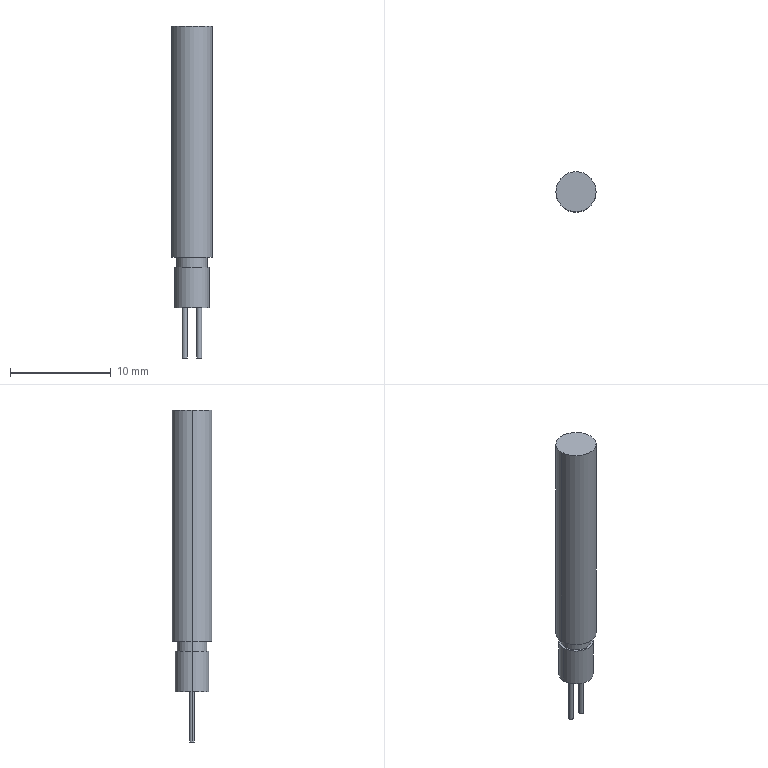Part | NX | 1 solid | 16 faces | box 4 x 4 x 33 mm | volume 334.375 mm3 | cylinder 10 | plane 6 | commonest cylinder face diameters 0.5 x4 3 x2 3.4 x2 4 x2
STEP:
#1=CARTESIAN_POINT('',(0.46,0.,-10.));
#2=VERTEX_POINT('',#1);
#3=CARTESIAN_POINT('',(0.96,0.,-10.));
#4=VERTEX_POINT('',#3);
#5=CARTESIAN_POINT('',(0.71,0.,-10.));
#6=DIRECTION('',(0.,0.,-1.));
#7=DIRECTION('',(-1.,0.,0.));
#8=AXIS2_PLACEMENT_3D('',#5,#6,#7);
#9=CIRCLE('',#8,0.25);
#10=EDGE_CURVE('',#2,#4,#9,.T.);
#11=ORIENTED_EDGE('',*,*,#10,.F.);
#12=CARTESIAN_POINT('',(0.46,0.,-5.));
#13=VERTEX_POINT('',#12);
#14=CARTESIAN_POINT('',(0.46,0.,-10.));
#15=DIRECTION('',(0.,0.,1.));
#16=VECTOR('',#15,1000.);
#17=LINE('',#14,#16);
#18=EDGE_CURVE('',#2,#13,#17,.T.);
#19=ORIENTED_EDGE('',*,*,#18,.T.);
#20=CARTESIAN_POINT('',(0.96,0.,-5.));
#21=VERTEX_POINT('',#20);
#22=CARTESIAN_POINT('',(0.71,0.,-5.));
#23=DIRECTION('',(0.,0.,-1.));
#24=DIRECTION('',(1.,0.,0.));
#25=AXIS2_PLACEMENT_3D('',#22,#23,#24);
#26=CIRCLE('',#25,0.25);
#27=EDGE_CURVE('',#13,#21,#26,.T.);
#28=ORIENTED_EDGE('',*,*,#27,.T.);
#29=CARTESIAN_POINT('',(0.96,0.,-10.));
#30=DIRECTION('',(0.,0.,1.));
#31=VECTOR('',#30,1000.);
#32=LINE('',#29,#31);
#33=EDGE_CURVE('',#4,#21,#32,.T.);
#34=ORIENTED_EDGE('',*,*,#33,.F.);
#35=EDGE_LOOP('',(#11,#19,#28,#34));
#36=FACE_BOUND('',#35,.T.);
#37=CARTESIAN_POINT('',(0.71,0.,-10.));
#38=DIRECTION('',(0.,0.,1.));
#39=DIRECTION('',(1.,0.,0.));
#40=AXIS2_PLACEMENT_3D('',#37,#38,#39);
#41=CYLINDRICAL_SURFACE('',#40,0.25);
#42=ADVANCED_FACE('',(#36),#41,.T.);
#43=CARTESIAN_POINT('',(-0.46,0.,-10.));
#44=VERTEX_POINT('',#43);
#45=CARTESIAN_POINT('',(-0.96,0.,-10.));
#46=VERTEX_POINT('',#45);
#47=CARTESIAN_POINT('',(-0.71,0.,-10.));
#48=DIRECTION('',(0.,0.,-1.));
#49=DIRECTION('',(1.,0.,0.));
#50=AXIS2_PLACEMENT_3D('',#47,#48,#49);
#51=CIRCLE('',#50,0.25);
#52=EDGE_CURVE('',#44,#46,#51,.T.);
#53=ORIENTED_EDGE('',*,*,#52,.F.);
#54=CARTESIAN_POINT('',(-0.46,0.,-5.));
#55=VERTEX_POINT('',#54);
#56=CARTESIAN_POINT('',(-0.46,0.,-10.));
#57=DIRECTION('',(0.,0.,1.));
#58=VECTOR('',#57,1000.);
#59=LINE('',#56,#58);
#60=EDGE_CURVE('',#44,#55,#59,.T.);
#61=ORIENTED_EDGE('',*,*,#60,.T.);
#62=CARTESIAN_POINT('',(-0.96,0.,-5.));
#63=VERTEX_POINT('',#62);
#64=CARTESIAN_POINT('',(-0.71,0.,-5.));
#65=DIRECTION('',(0.,0.,-1.));
#66=DIRECTION('',(1.,0.,0.));
#67=AXIS2_PLACEMENT_3D('',#64,#65,#66);
#68=CIRCLE('',#67,0.25);
#69=EDGE_CURVE('',#55,#63,#68,.T.);
#70=ORIENTED_EDGE('',*,*,#69,.T.);
#71=CARTESIAN_POINT('',(-0.96,0.,-10.));
#72=DIRECTION('',(0.,0.,1.));
#73=VECTOR('',#72,1000.);
#74=LINE('',#71,#73);
#75=EDGE_CURVE('',#46,#63,#74,.T.);
#76=ORIENTED_EDGE('',*,*,#75,.F.);
#77=EDGE_LOOP('',(#53,#61,#70,#76));
#78=FACE_BOUND('',#77,.T.);
#79=CARTESIAN_POINT('',(-0.71,0.,-10.));
#80=DIRECTION('',(0.,0.,1.));
#81=DIRECTION('',(1.,0.,0.));
#82=AXIS2_PLACEMENT_3D('',#79,#80,#81);
#83=CYLINDRICAL_SURFACE('',#82,0.25);
#84=ADVANCED_FACE('',(#78),#83,.T.);
#85=CARTESIAN_POINT('',(1.7,0.,-1.));
#86=VERTEX_POINT('',#85);
#87=CARTESIAN_POINT('',(-1.7,0.,-1.));
#88=VERTEX_POINT('',#87);
#89=CARTESIAN_POINT('',(0.,0.,-1.));
#90=DIRECTION('',(0.,0.,-1.));
#91=DIRECTION('',(-1.,0.,0.));
#92=AXIS2_PLACEMENT_3D('',#89,#90,#91);
#93=CIRCLE('',#92,1.7);
#94=EDGE_CURVE('',#86,#88,#93,.T.);
#95=ORIENTED_EDGE('',*,*,#94,.T.);
#96=CARTESIAN_POINT('',(-1.7,0.,-5.));
#97=VERTEX_POINT('',#96);
#98=CARTESIAN_POINT('',(-1.7,0.,-5.));
#99=DIRECTION('',(0.,0.,1.));
#100=VECTOR('',#99,1000.);
#101=LINE('',#98,#100);
#102=EDGE_CURVE('',#97,#88,#101,.T.);
#103=ORIENTED_EDGE('',*,*,#102,.F.);
#104=CARTESIAN_POINT('',(1.7,0.,-5.));
#105=VERTEX_POINT('',#104);
#106=CARTESIAN_POINT('',(0.,0.,-5.));
#107=DIRECTION('',(0.,0.,-1.));
#108=DIRECTION('',(-1.,0.,0.));
#109=AXIS2_PLACEMENT_3D('',#106,#107,#108);
#110=CIRCLE('',#109,1.7);
#111=EDGE_CURVE('',#105,#97,#110,.T.);
#112=ORIENTED_EDGE('',*,*,#111,.F.);
#113=CARTESIAN_POINT('',(1.7,0.,-5.));
#114=DIRECTION('',(0.,0.,1.));
#115=VECTOR('',#114,1000.);
#116=LINE('',#113,#115);
#117=EDGE_CURVE('',#105,#86,#116,.T.);
#118=ORIENTED_EDGE('',*,*,#117,.T.);
#119=EDGE_LOOP('',(#95,#103,#112,#118));
#120=FACE_BOUND('',#119,.T.);
#121=CARTESIAN_POINT('',(0.,0.,-5.));
#122=DIRECTION('',(0.,0.,1.));
#123=DIRECTION('',(1.,0.,0.));
#124=AXIS2_PLACEMENT_3D('',#121,#122,#123);
#125=CYLINDRICAL_SURFACE('',#124,1.7);
#126=ADVANCED_FACE('',(#120),#125,.T.);
#127=CARTESIAN_POINT('',(2.,0.,23.));
#128=VERTEX_POINT('',#127);
#129=CARTESIAN_POINT('',(-2.,0.,23.));
#130=VERTEX_POINT('',#129);
#131=CARTESIAN_POINT('',(0.,0.,23.));
#132=DIRECTION('',(0.,0.,1.));
#133=DIRECTION('',(1.,0.,0.));
#134=AXIS2_PLACEMENT_3D('',#131,#132,#133);
#135=CIRCLE('',#134,2.);
#136=EDGE_CURVE('',#128,#130,#135,.T.);
#137=ORIENTED_EDGE('',*,*,#136,.F.);
#138=CARTESIAN_POINT('',(2.,0.,0.));
#139=VERTEX_POINT('',#138);
#140=CARTESIAN_POINT('',(2.,0.,23.));
#141=DIRECTION('',(0.,0.,-1.));
#142=VECTOR('',#141,1000.);
#143=LINE('',#140,#142);
#144=EDGE_CURVE('',#128,#139,#143,.T.);
#145=ORIENTED_EDGE('',*,*,#144,.T.);
#146=CARTESIAN_POINT('',(-2.,0.,0.));
#147=VERTEX_POINT('',#146);
#148=CARTESIAN_POINT('',(0.,0.,0.));
#149=DIRECTION('',(0.,0.,1.));
#150=DIRECTION('',(1.,0.,0.));
#151=AXIS2_PLACEMENT_3D('',#148,#149,#150);
#152=CIRCLE('',#151,2.);
#153=EDGE_CURVE('',#139,#147,#152,.T.);
#154=ORIENTED_EDGE('',*,*,#153,.T.);
#155=CARTESIAN_POINT('',(-2.,0.,23.));
#156=DIRECTION('',(0.,0.,-1.));
#157=VECTOR('',#156,1000.);
#158=LINE('',#155,#157);
#159=EDGE_CURVE('',#130,#147,#158,.T.);
#160=ORIENTED_EDGE('',*,*,#159,.F.);
#161=EDGE_LOOP('',(#137,#145,#154,#160));
#162=FACE_BOUND('',#161,.T.);
#163=CARTESIAN_POINT('',(0.,0.,23.));
#164=DIRECTION('',(0.,0.,-1.));
#165=DIRECTION('',(-1.,0.,0.));
#166=AXIS2_PLACEMENT_3D('',#163,#164,#165);
#167=CYLINDRICAL_SURFACE('',#166,2.);
#168=ADVANCED_FACE('',(#162),#167,.T.);
#169=CARTESIAN_POINT('',(-1.5,0.,-1.));
#170=VERTEX_POINT('',#169);
#171=CARTESIAN_POINT('',(1.5,0.,-1.));
#172=VERTEX_POINT('',#171);
#173=CARTESIAN_POINT('',(0.,0.,-1.));
#174=DIRECTION('',(0.,0.,-1.));
#175=DIRECTION('',(-1.,0.,0.));
#176=AXIS2_PLACEMENT_3D('',#173,#174,#175);
#177=CIRCLE('',#176,1.5);
#178=EDGE_CURVE('',#170,#172,#177,.T.);
#179=ORIENTED_EDGE('',*,*,#178,.F.);
#180=CARTESIAN_POINT('',(-1.5,0.,0.));
#181=VERTEX_POINT('',#180);
#182=CARTESIAN_POINT('',(-1.5,0.,-1.));
#183=DIRECTION('',(0.,0.,1.));
#184=VECTOR('',#183,1000.);
#185=LINE('',#182,#184);
#186=EDGE_CURVE('',#170,#181,#185,.T.);
#187=ORIENTED_EDGE('',*,*,#186,.T.);
#188=CARTESIAN_POINT('',(1.5,0.,0.));
#189=VERTEX_POINT('',#188);
#190=CARTESIAN_POINT('',(0.,0.,0.));
#191=DIRECTION('',(0.,0.,-1.));
#192=DIRECTION('',(1.,0.,0.));
#193=AXIS2_PLACEMENT_3D('',#190,#191,#192);
#194=CIRCLE('',#193,1.5);
#195=EDGE_CURVE('',#181,#189,#194,.T.);
#196=ORIENTED_EDGE('',*,*,#195,.T.);
#197=CARTESIAN_POINT('',(1.5,0.,-1.));
#198=DIRECTION('',(0.,0.,1.));
#199=VECTOR('',#198,1000.);
#200=LINE('',#197,#199);
#201=EDGE_CURVE('',#172,#189,#200,.T.);
#202=ORIENTED_EDGE('',*,*,#201,.F.);
#203=EDGE_LOOP('',(#179,#187,#196,#202));
#204=FACE_BOUND('',#203,.T.);
#205=CARTESIAN_POINT('',(0.,0.,-1.));
#206=DIRECTION('',(0.,0.,1.));
#207=DIRECTION('',(1.,0.,0.));
#208=AXIS2_PLACEMENT_3D('',#205,#206,#207);
#209=CYLINDRICAL_SURFACE('',#208,1.5);
#210=ADVANCED_FACE('',(#204),#209,.T.);
#211=ORIENTED_EDGE('',*,*,#111,.T.);
#212=CARTESIAN_POINT('',(0.,0.,-5.));
#213=DIRECTION('',(0.,0.,-1.));
#214=DIRECTION('',(-1.,0.,0.));
#215=AXIS2_PLACEMENT_3D('',#212,#213,#214);
#216=CIRCLE('',#215,1.7);
#217=EDGE_CURVE('',#97,#105,#216,.T.);
#218=ORIENTED_EDGE('',*,*,#217,.T.);
#219=EDGE_LOOP('',(#211,#218));
#220=FACE_BOUND('',#219,.T.);
#221=ORIENTED_EDGE('',*,*,#27,.F.);
#222=CARTESIAN_POINT('',(0.71,0.,-5.));
#223=DIRECTION('',(0.,0.,-1.));
#224=DIRECTION('',(1.,0.,0.));
#225=AXIS2_PLACEMENT_3D('',#222,#223,#224);
#226=CIRCLE('',#225,0.25);
#227=EDGE_CURVE('',#21,#13,#226,.T.);
#228=ORIENTED_EDGE('',*,*,#227,.F.);
#229=EDGE_LOOP('',(#221,#228));
#230=FACE_BOUND('',#229,.T.);
#231=ORIENTED_EDGE('',*,*,#69,.F.);
#232=CARTESIAN_POINT('',(-0.71,0.,-5.));
#233=DIRECTION('',(0.,0.,-1.));
#234=DIRECTION('',(1.,0.,0.));
#235=AXIS2_PLACEMENT_3D('',#232,#233,#234);
#236=CIRCLE('',#235,0.25);
#237=EDGE_CURVE('',#63,#55,#236,.T.);
#238=ORIENTED_EDGE('',*,*,#237,.F.);
#239=EDGE_LOOP('',(#231,#238));
#240=FACE_BOUND('',#239,.T.);
#241=CARTESIAN_POINT('',(0.71,0.,-5.));
#242=DIRECTION('',(0.,0.,1.));
#243=DIRECTION('',(1.,0.,0.));
#244=AXIS2_PLACEMENT_3D('',#241,#242,#243);
#245=PLANE('',#244);
#246=ADVANCED_FACE('',(#220,#230,#240),#245,.F.);
#247=ORIENTED_EDGE('',*,*,#136,.T.);
#248=CARTESIAN_POINT('',(0.,0.,23.));
#249=DIRECTION('',(0.,0.,1.));
#250=DIRECTION('',(1.,0.,0.));
#251=AXIS2_PLACEMENT_3D('',#248,#249,#250);
#252=CIRCLE('',#251,2.);
#253=EDGE_CURVE('',#130,#128,#252,.T.);
#254=ORIENTED_EDGE('',*,*,#253,.T.);
#255=EDGE_LOOP('',(#247,#254));
#256=FACE_BOUND('',#255,.T.);
#257=CARTESIAN_POINT('',(0.,0.,23.));
#258=DIRECTION('',(0.,0.,1.));
#259=DIRECTION('',(1.,0.,0.));
#260=AXIS2_PLACEMENT_3D('',#257,#258,#259);
#261=PLANE('',#260);
#262=ADVANCED_FACE('',(#256),#261,.T.);
#263=ORIENTED_EDGE('',*,*,#52,.T.);
#264=CARTESIAN_POINT('',(-0.71,0.,-10.));
#265=DIRECTION('',(0.,0.,-1.));
#266=DIRECTION('',(1.,0.,0.));
#267=AXIS2_PLACEMENT_3D('',#264,#265,#266);
#268=CIRCLE('',#267,0.25);
#269=EDGE_CURVE('',#46,#44,#268,.T.);
#270=ORIENTED_EDGE('',*,*,#269,.T.);
#271=EDGE_LOOP('',(#263,#270));
#272=FACE_BOUND('',#271,.T.);
#273=CARTESIAN_POINT('',(-0.71,0.,-10.));
#274=DIRECTION('',(0.,0.,1.));
#275=DIRECTION('',(1.,0.,0.));
#276=AXIS2_PLACEMENT_3D('',#273,#274,#275);
#277=PLANE('',#276);
#278=ADVANCED_FACE('',(#272),#277,.F.);
#279=CARTESIAN_POINT('',(0.,0.,0.));
#280=DIRECTION('',(0.,0.,1.));
#281=DIRECTION('',(1.,0.,0.));
#282=AXIS2_PLACEMENT_3D('',#279,#280,#281);
#283=CIRCLE('',#282,2.);
#284=EDGE_CURVE('',#147,#139,#283,.T.);
#285=ORIENTED_EDGE('',*,*,#284,.F.);
#286=ORIENTED_EDGE('',*,*,#153,.F.);
#287=EDGE_LOOP('',(#285,#286));
#288=FACE_BOUND('',#287,.T.);
#289=ORIENTED_EDGE('',*,*,#195,.F.);
#290=CARTESIAN_POINT('',(0.,0.,0.));
#291=DIRECTION('',(0.,0.,-1.));
#292=DIRECTION('',(1.,0.,0.));
#293=AXIS2_PLACEMENT_3D('',#290,#291,#292);
#294=CIRCLE('',#293,1.5);
#295=EDGE_CURVE('',#189,#181,#294,.T.);
#296=ORIENTED_EDGE('',*,*,#295,.F.);
#297=EDGE_LOOP('',(#289,#296));
#298=FACE_BOUND('',#297,.T.);
#299=CARTESIAN_POINT('',(0.,0.,0.));
#300=DIRECTION('',(0.,0.,1.));
#301=DIRECTION('',(1.,0.,0.));
#302=AXIS2_PLACEMENT_3D('',#299,#300,#301);
#303=PLANE('',#302);
#304=ADVANCED_FACE('',(#288,#298),#303,.F.);
#305=ORIENTED_EDGE('',*,*,#94,.F.);
#306=CARTESIAN_POINT('',(0.,0.,-1.));
#307=DIRECTION('',(0.,0.,-1.));
#308=DIRECTION('',(-1.,0.,0.));
#309=AXIS2_PLACEMENT_3D('',#306,#307,#308);
#310=CIRCLE('',#309,1.7);
#311=EDGE_CURVE('',#88,#86,#310,.T.);
#312=ORIENTED_EDGE('',*,*,#311,.F.);
#313=EDGE_LOOP('',(#305,#312));
#314=FACE_BOUND('',#313,.T.);
#315=ORIENTED_EDGE('',*,*,#178,.T.);
#316=CARTESIAN_POINT('',(0.,0.,-1.));
#317=DIRECTION('',(0.,0.,-1.));
#318=DIRECTION('',(-1.,0.,0.));
#319=AXIS2_PLACEMENT_3D('',#316,#317,#318);
#320=CIRCLE('',#319,1.5);
#321=EDGE_CURVE('',#172,#170,#320,.T.);
#322=ORIENTED_EDGE('',*,*,#321,.T.);
#323=EDGE_LOOP('',(#315,#322));
#324=FACE_BOUND('',#323,.T.);
#325=CARTESIAN_POINT('',(0.,0.,-1.));
#326=DIRECTION('',(0.,0.,-1.));
#327=DIRECTION('',(0.,-1.,0.));
#328=AXIS2_PLACEMENT_3D('',#325,#326,#327);
#329=PLANE('',#328);
#330=ADVANCED_FACE('',(#314,#324),#329,.F.);
#331=ORIENTED_EDGE('',*,*,#10,.T.);
#332=CARTESIAN_POINT('',(0.71,0.,-10.));
#333=DIRECTION('',(0.,0.,-1.));
#334=DIRECTION('',(-1.,0.,0.));
#335=AXIS2_PLACEMENT_3D('',#332,#333,#334);
#336=CIRCLE('',#335,0.25);
#337=EDGE_CURVE('',#4,#2,#336,.T.);
#338=ORIENTED_EDGE('',*,*,#337,.T.);
#339=EDGE_LOOP('',(#331,#338));
#340=FACE_BOUND('',#339,.T.);
#341=CARTESIAN_POINT('',(0.71,0.,-10.));
#342=DIRECTION('',(0.,0.,-1.));
#343=DIRECTION('',(0.,-1.,0.));
#344=AXIS2_PLACEMENT_3D('',#341,#342,#343);
#345=PLANE('',#344);
#346=ADVANCED_FACE('',(#340),#345,.T.);
#347=ORIENTED_EDGE('',*,*,#60,.F.);
#348=ORIENTED_EDGE('',*,*,#269,.F.);
#349=ORIENTED_EDGE('',*,*,#75,.T.);
#350=ORIENTED_EDGE('',*,*,#237,.T.);
#351=EDGE_LOOP('',(#347,#348,#349,#350));
#352=FACE_BOUND('',#351,.T.);
#353=CARTESIAN_POINT('',(-0.71,0.,-10.));
#354=DIRECTION('',(0.,0.,1.));
#355=DIRECTION('',(1.,0.,0.));
#356=AXIS2_PLACEMENT_3D('',#353,#354,#355);
#357=CYLINDRICAL_SURFACE('',#356,0.25);
#358=ADVANCED_FACE('',(#352),#357,.T.);
#359=ORIENTED_EDGE('',*,*,#117,.F.);
#360=ORIENTED_EDGE('',*,*,#217,.F.);
#361=ORIENTED_EDGE('',*,*,#102,.T.);
#362=ORIENTED_EDGE('',*,*,#311,.T.);
#363=EDGE_LOOP('',(#359,#360,#361,#362));
#364=FACE_BOUND('',#363,.T.);
#365=CARTESIAN_POINT('',(0.,0.,-5.));
#366=DIRECTION('',(0.,0.,1.));
#367=DIRECTION('',(1.,0.,0.));
#368=AXIS2_PLACEMENT_3D('',#365,#366,#367);
#369=CYLINDRICAL_SURFACE('',#368,1.7);
#370=ADVANCED_FACE('',(#364),#369,.T.);
#371=ORIENTED_EDGE('',*,*,#33,.T.);
#372=ORIENTED_EDGE('',*,*,#227,.T.);
#373=ORIENTED_EDGE('',*,*,#18,.F.);
#374=ORIENTED_EDGE('',*,*,#337,.F.);
#375=EDGE_LOOP('',(#371,#372,#373,#374));
#376=FACE_BOUND('',#375,.T.);
#377=CARTESIAN_POINT('',(0.71,0.,-10.));
#378=DIRECTION('',(0.,0.,1.));
#379=DIRECTION('',(1.,0.,0.));
#380=AXIS2_PLACEMENT_3D('',#377,#378,#379);
#381=CYLINDRICAL_SURFACE('',#380,0.25);
#382=ADVANCED_FACE('',(#376),#381,.T.);
#383=ORIENTED_EDGE('',*,*,#284,.T.);
#384=ORIENTED_EDGE('',*,*,#144,.F.);
#385=ORIENTED_EDGE('',*,*,#253,.F.);
#386=ORIENTED_EDGE('',*,*,#159,.T.);
#387=EDGE_LOOP('',(#383,#384,#385,#386));
#388=FACE_BOUND('',#387,.T.);
#389=CARTESIAN_POINT('',(0.,0.,23.));
#390=DIRECTION('',(0.,0.,-1.));
#391=DIRECTION('',(-1.,0.,0.));
#392=AXIS2_PLACEMENT_3D('',#389,#390,#391);
#393=CYLINDRICAL_SURFACE('',#392,2.);
#394=ADVANCED_FACE('',(#388),#393,.T.);
#395=ORIENTED_EDGE('',*,*,#201,.T.);
#396=ORIENTED_EDGE('',*,*,#295,.T.);
#397=ORIENTED_EDGE('',*,*,#186,.F.);
#398=ORIENTED_EDGE('',*,*,#321,.F.);
#399=EDGE_LOOP('',(#395,#396,#397,#398));
#400=FACE_BOUND('',#399,.T.);
#401=CARTESIAN_POINT('',(0.,0.,-1.));
#402=DIRECTION('',(0.,0.,1.));
#403=DIRECTION('',(1.,0.,0.));
#404=AXIS2_PLACEMENT_3D('',#401,#402,#403);
#405=CYLINDRICAL_SURFACE('',#404,1.5);
#406=ADVANCED_FACE('',(#400),#405,.T.);
#407=CLOSED_SHELL('',(#42,#84,#126,#168,#210,#246,#262,#278,#304,#330,#346,#358,#370,#382,#394,#406));
#408=MANIFOLD_SOLID_BREP('',#407);
#409=(LENGTH_UNIT()NAMED_UNIT(*)SI_UNIT(.MILLI.,.METRE.));
#410=UNCERTAINTY_MEASURE_WITH_UNIT(LENGTH_MEASURE(0.00001),#409,'','');
#411=(NAMED_UNIT(*)PLANE_ANGLE_UNIT()SI_UNIT($,.RADIAN.));
#412=(NAMED_UNIT(*)SI_UNIT($,.STERADIAN.)SOLID_ANGLE_UNIT());
#413=(GEOMETRIC_REPRESENTATION_CONTEXT(3)GLOBAL_UNCERTAINTY_ASSIGNED_CONTEXT((#410))GLOBAL_UNIT_ASSIGNED_CONTEXT((#409,#411,#412))REPRESENTATION_CONTEXT('',''));
#414=ADVANCED_BREP_SHAPE_REPRESENTATION('',(#408),#413);